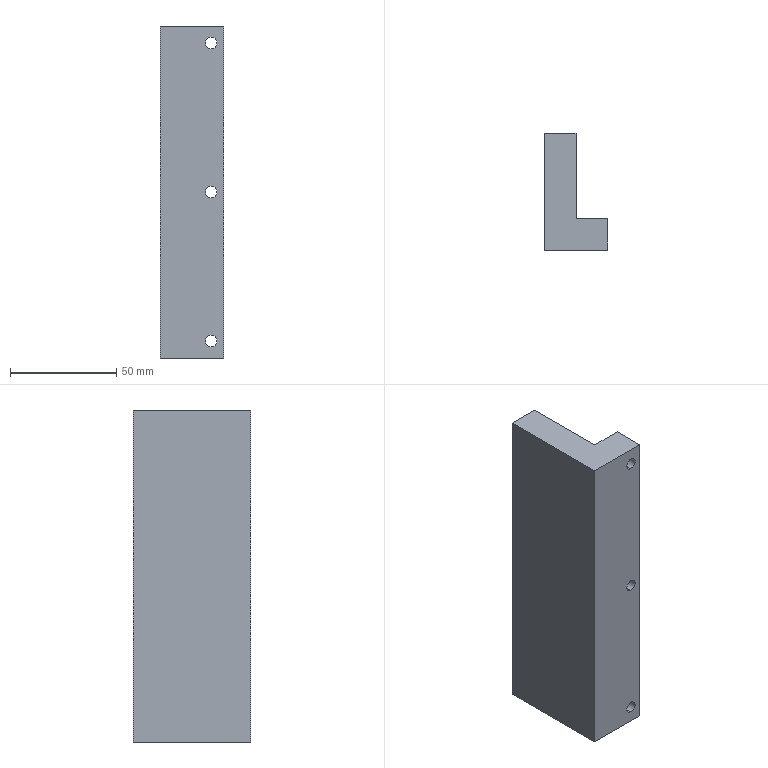Part | SolidWorks | features 3DProfileFeature 1, Cut 1, Extrusion 1, HoleWzd 1 | 1 solid | 26 faces | box 30 x 55 x 156 mm | volume 162115 mm3 | cylinder 12 | plane 8 | cone 6 | commonest cylinder face diameters 4.2 x6 5.5 x6
STEP:
#1=CARTESIAN_POINT('',(24.,0.,67.25));
#2=VERTEX_POINT('',#1);
#3=CARTESIAN_POINT('',(24.,0.,72.75));
#4=VERTEX_POINT('',#3);
#5=CARTESIAN_POINT('',(24.,0.,70.));
#6=DIRECTION('',(0.,1.,0.));
#7=DIRECTION('',(0.,0.,-1.));
#8=AXIS2_PLACEMENT_3D('',#5,#6,#7);
#9=CIRCLE('',#8,2.75);
#10=EDGE_CURVE('',#2,#4,#9,.T.);
#11=ORIENTED_EDGE('',*,*,#10,.F.);
#12=CARTESIAN_POINT('',(24.,15.,67.25));
#13=VERTEX_POINT('',#12);
#14=CARTESIAN_POINT('',(24.,0.,67.25));
#15=DIRECTION('',(0.,1.,0.));
#16=VECTOR('',#15,1000.);
#17=LINE('',#14,#16);
#18=EDGE_CURVE('',#2,#13,#17,.T.);
#19=ORIENTED_EDGE('',*,*,#18,.T.);
#20=CARTESIAN_POINT('',(24.,15.,72.75));
#21=VERTEX_POINT('',#20);
#22=CARTESIAN_POINT('',(24.,15.,70.));
#23=DIRECTION('',(0.,1.,0.));
#24=DIRECTION('',(0.,0.,-1.));
#25=AXIS2_PLACEMENT_3D('',#22,#23,#24);
#26=CIRCLE('',#25,2.75);
#27=EDGE_CURVE('',#13,#21,#26,.T.);
#28=ORIENTED_EDGE('',*,*,#27,.T.);
#29=CARTESIAN_POINT('',(24.,0.,72.75));
#30=DIRECTION('',(0.,1.,0.));
#31=VECTOR('',#30,1000.);
#32=LINE('',#29,#31);
#33=EDGE_CURVE('',#4,#21,#32,.T.);
#34=ORIENTED_EDGE('',*,*,#33,.F.);
#35=EDGE_LOOP('',(#11,#19,#28,#34));
#36=FACE_OUTER_BOUND('',#35,.T.);
#37=CARTESIAN_POINT('',(24.,0.,70.));
#38=DIRECTION('',(0.,1.,0.));
#39=DIRECTION('',(0.,0.,1.));
#40=AXIS2_PLACEMENT_3D('',#37,#38,#39);
#41=CYLINDRICAL_SURFACE('',#40,2.75);
#42=ADVANCED_FACE('',(#36),#41,.F.);
#43=CARTESIAN_POINT('',(24.,0.,-72.75));
#44=VERTEX_POINT('',#43);
#45=CARTESIAN_POINT('',(24.,0.,-67.25));
#46=VERTEX_POINT('',#45);
#47=CARTESIAN_POINT('',(24.,0.,-70.));
#48=DIRECTION('',(0.,1.,0.));
#49=DIRECTION('',(0.,0.,1.));
#50=AXIS2_PLACEMENT_3D('',#47,#48,#49);
#51=CIRCLE('',#50,2.75);
#52=EDGE_CURVE('',#44,#46,#51,.T.);
#53=ORIENTED_EDGE('',*,*,#52,.F.);
#54=CARTESIAN_POINT('',(24.,15.,-72.75));
#55=VERTEX_POINT('',#54);
#56=CARTESIAN_POINT('',(24.,0.,-72.75));
#57=DIRECTION('',(0.,1.,0.));
#58=VECTOR('',#57,1000.);
#59=LINE('',#56,#58);
#60=EDGE_CURVE('',#44,#55,#59,.T.);
#61=ORIENTED_EDGE('',*,*,#60,.T.);
#62=CARTESIAN_POINT('',(24.,15.,-67.25));
#63=VERTEX_POINT('',#62);
#64=CARTESIAN_POINT('',(24.,15.,-70.));
#65=DIRECTION('',(0.,1.,0.));
#66=DIRECTION('',(0.,0.,1.));
#67=AXIS2_PLACEMENT_3D('',#64,#65,#66);
#68=CIRCLE('',#67,2.75);
#69=EDGE_CURVE('',#55,#63,#68,.T.);
#70=ORIENTED_EDGE('',*,*,#69,.T.);
#71=CARTESIAN_POINT('',(24.,0.,-67.25));
#72=DIRECTION('',(0.,1.,0.));
#73=VECTOR('',#72,1000.);
#74=LINE('',#71,#73);
#75=EDGE_CURVE('',#46,#63,#74,.T.);
#76=ORIENTED_EDGE('',*,*,#75,.F.);
#77=EDGE_LOOP('',(#53,#61,#70,#76));
#78=FACE_OUTER_BOUND('',#77,.T.);
#79=CARTESIAN_POINT('',(24.,0.,-70.));
#80=DIRECTION('',(0.,1.,0.));
#81=DIRECTION('',(0.,0.,1.));
#82=AXIS2_PLACEMENT_3D('',#79,#80,#81);
#83=CYLINDRICAL_SURFACE('',#82,2.75);
#84=ADVANCED_FACE('',(#78),#83,.F.);
#85=CARTESIAN_POINT('',(24.,0.,-2.75));
#86=VERTEX_POINT('',#85);
#87=CARTESIAN_POINT('',(24.,0.,2.75));
#88=VERTEX_POINT('',#87);
#89=CARTESIAN_POINT('',(24.,0.,0.));
#90=DIRECTION('',(0.,1.,0.));
#91=DIRECTION('',(0.,0.,1.));
#92=AXIS2_PLACEMENT_3D('',#89,#90,#91);
#93=CIRCLE('',#92,2.75);
#94=EDGE_CURVE('',#86,#88,#93,.T.);
#95=ORIENTED_EDGE('',*,*,#94,.F.);
#96=CARTESIAN_POINT('',(24.,15.,-2.75));
#97=VERTEX_POINT('',#96);
#98=CARTESIAN_POINT('',(24.,0.,-2.75));
#99=DIRECTION('',(0.,1.,0.));
#100=VECTOR('',#99,1000.);
#101=LINE('',#98,#100);
#102=EDGE_CURVE('',#86,#97,#101,.T.);
#103=ORIENTED_EDGE('',*,*,#102,.T.);
#104=CARTESIAN_POINT('',(24.,15.,2.75));
#105=VERTEX_POINT('',#104);
#106=CARTESIAN_POINT('',(24.,15.,0.));
#107=DIRECTION('',(0.,1.,0.));
#108=DIRECTION('',(0.,0.,1.));
#109=AXIS2_PLACEMENT_3D('',#106,#107,#108);
#110=CIRCLE('',#109,2.75);
#111=EDGE_CURVE('',#97,#105,#110,.T.);
#112=ORIENTED_EDGE('',*,*,#111,.T.);
#113=CARTESIAN_POINT('',(24.,0.,2.75));
#114=DIRECTION('',(0.,1.,0.));
#115=VECTOR('',#114,1000.);
#116=LINE('',#113,#115);
#117=EDGE_CURVE('',#88,#105,#116,.T.);
#118=ORIENTED_EDGE('',*,*,#117,.F.);
#119=EDGE_LOOP('',(#95,#103,#112,#118));
#120=FACE_OUTER_BOUND('',#119,.T.);
#121=CARTESIAN_POINT('',(24.,0.,0.));
#122=DIRECTION('',(0.,1.,0.));
#123=DIRECTION('',(0.,0.,1.));
#124=AXIS2_PLACEMENT_3D('',#121,#122,#123);
#125=CYLINDRICAL_SURFACE('',#124,2.75);
#126=ADVANCED_FACE('',(#120),#125,.F.);
#127=CARTESIAN_POINT('',(7.5,39.338,0.));
#128=VERTEX_POINT('',#127);
#129=CARTESIAN_POINT('',(7.5,40.6,2.1));
#130=VERTEX_POINT('',#129);
#131=CARTESIAN_POINT('',(7.5,40.6,2.1));
#132=DIRECTION('',(0.,0.515,0.8572));
#133=VECTOR('',#132,1000.);
#134=LINE('',#131,#133);
#135=EDGE_CURVE('',#128,#130,#134,.T.);
#136=ORIENTED_EDGE('',*,*,#135,.F.);
#137=CARTESIAN_POINT('',(7.5,40.6,-2.1));
#138=VERTEX_POINT('',#137);
#139=CARTESIAN_POINT('',(7.5,40.6,-2.1));
#140=DIRECTION('',(0.,0.515,-0.8572));
#141=VECTOR('',#140,1000.);
#142=LINE('',#139,#141);
#143=EDGE_CURVE('',#128,#138,#142,.T.);
#144=ORIENTED_EDGE('',*,*,#143,.T.);
#145=CARTESIAN_POINT('',(7.5,40.6,0.));
#146=DIRECTION('',(0.,1.,0.));
#147=DIRECTION('',(0.,0.,1.));
#148=AXIS2_PLACEMENT_3D('',#145,#146,#147);
#149=CIRCLE('',#148,2.1);
#150=EDGE_CURVE('',#138,#130,#149,.T.);
#151=ORIENTED_EDGE('',*,*,#150,.T.);
#152=EDGE_LOOP('',(#136,#144,#151));
#153=FACE_OUTER_BOUND('',#152,.T.);
#154=CARTESIAN_POINT('',(7.5,40.6,0.));
#155=DIRECTION('',(0.,1.,0.));
#156=DIRECTION('',(0.,0.,1.));
#157=AXIS2_PLACEMENT_3D('',#154,#155,#156);
#158=CONICAL_SURFACE('',#157,2.1,1.03);
#159=ADVANCED_FACE('',(#153),#158,.F.);
#160=ORIENTED_EDGE('',*,*,#150,.F.);
#161=CARTESIAN_POINT('',(7.5,55.,-2.1));
#162=VERTEX_POINT('',#161);
#163=CARTESIAN_POINT('',(7.5,55.,-2.1));
#164=DIRECTION('',(0.,1.,0.));
#165=VECTOR('',#164,1000.);
#166=LINE('',#163,#165);
#167=EDGE_CURVE('',#138,#162,#166,.T.);
#168=ORIENTED_EDGE('',*,*,#167,.T.);
#169=CARTESIAN_POINT('',(7.5,55.,2.1));
#170=VERTEX_POINT('',#169);
#171=CARTESIAN_POINT('',(7.5,55.,0.));
#172=DIRECTION('',(0.,1.,0.));
#173=DIRECTION('',(0.,0.,1.));
#174=AXIS2_PLACEMENT_3D('',#171,#172,#173);
#175=CIRCLE('',#174,2.1);
#176=EDGE_CURVE('',#162,#170,#175,.T.);
#177=ORIENTED_EDGE('',*,*,#176,.T.);
#178=CARTESIAN_POINT('',(7.5,55.,2.1));
#179=DIRECTION('',(0.,1.,0.));
#180=VECTOR('',#179,1000.);
#181=LINE('',#178,#180);
#182=EDGE_CURVE('',#130,#170,#181,.T.);
#183=ORIENTED_EDGE('',*,*,#182,.F.);
#184=EDGE_LOOP('',(#160,#168,#177,#183));
#185=FACE_OUTER_BOUND('',#184,.T.);
#186=CARTESIAN_POINT('',(7.5,55.,0.));
#187=DIRECTION('',(0.,1.,0.));
#188=DIRECTION('',(0.,0.,1.));
#189=AXIS2_PLACEMENT_3D('',#186,#187,#188);
#190=CYLINDRICAL_SURFACE('',#189,2.1);
#191=ADVANCED_FACE('',(#185),#190,.F.);
#192=CARTESIAN_POINT('',(7.5,39.338,-70.));
#193=VERTEX_POINT('',#192);
#194=CARTESIAN_POINT('',(7.5,40.6,-67.9));
#195=VERTEX_POINT('',#194);
#196=CARTESIAN_POINT('',(7.5,40.6,-67.9));
#197=DIRECTION('',(0.,0.515,0.8572));
#198=VECTOR('',#197,1000.);
#199=LINE('',#196,#198);
#200=EDGE_CURVE('',#193,#195,#199,.T.);
#201=ORIENTED_EDGE('',*,*,#200,.F.);
#202=CARTESIAN_POINT('',(7.5,40.6,-72.1));
#203=VERTEX_POINT('',#202);
#204=CARTESIAN_POINT('',(7.5,40.6,-72.1));
#205=DIRECTION('',(0.,0.515,-0.8572));
#206=VECTOR('',#205,1000.);
#207=LINE('',#204,#206);
#208=EDGE_CURVE('',#193,#203,#207,.T.);
#209=ORIENTED_EDGE('',*,*,#208,.T.);
#210=CARTESIAN_POINT('',(7.5,40.6,-70.));
#211=DIRECTION('',(0.,1.,0.));
#212=DIRECTION('',(0.,0.,1.));
#213=AXIS2_PLACEMENT_3D('',#210,#211,#212);
#214=CIRCLE('',#213,2.1);
#215=EDGE_CURVE('',#203,#195,#214,.T.);
#216=ORIENTED_EDGE('',*,*,#215,.T.);
#217=EDGE_LOOP('',(#201,#209,#216));
#218=FACE_OUTER_BOUND('',#217,.T.);
#219=CARTESIAN_POINT('',(7.5,40.6,-70.));
#220=DIRECTION('',(0.,1.,0.));
#221=DIRECTION('',(0.,0.,1.));
#222=AXIS2_PLACEMENT_3D('',#219,#220,#221);
#223=CONICAL_SURFACE('',#222,2.1,1.03);
#224=ADVANCED_FACE('',(#218),#223,.F.);
#225=ORIENTED_EDGE('',*,*,#215,.F.);
#226=CARTESIAN_POINT('',(7.5,55.,-72.1));
#227=VERTEX_POINT('',#226);
#228=CARTESIAN_POINT('',(7.5,55.,-72.1));
#229=DIRECTION('',(0.,1.,0.));
#230=VECTOR('',#229,1000.);
#231=LINE('',#228,#230);
#232=EDGE_CURVE('',#203,#227,#231,.T.);
#233=ORIENTED_EDGE('',*,*,#232,.T.);
#234=CARTESIAN_POINT('',(7.5,55.,-67.9));
#235=VERTEX_POINT('',#234);
#236=CARTESIAN_POINT('',(7.5,55.,-70.));
#237=DIRECTION('',(0.,1.,0.));
#238=DIRECTION('',(0.,0.,1.));
#239=AXIS2_PLACEMENT_3D('',#236,#237,#238);
#240=CIRCLE('',#239,2.1);
#241=EDGE_CURVE('',#227,#235,#240,.T.);
#242=ORIENTED_EDGE('',*,*,#241,.T.);
#243=CARTESIAN_POINT('',(7.5,55.,-67.9));
#244=DIRECTION('',(0.,1.,0.));
#245=VECTOR('',#244,1000.);
#246=LINE('',#243,#245);
#247=EDGE_CURVE('',#195,#235,#246,.T.);
#248=ORIENTED_EDGE('',*,*,#247,.F.);
#249=EDGE_LOOP('',(#225,#233,#242,#248));
#250=FACE_OUTER_BOUND('',#249,.T.);
#251=CARTESIAN_POINT('',(7.5,55.,-70.));
#252=DIRECTION('',(0.,1.,0.));
#253=DIRECTION('',(0.,0.,1.));
#254=AXIS2_PLACEMENT_3D('',#251,#252,#253);
#255=CYLINDRICAL_SURFACE('',#254,2.1);
#256=ADVANCED_FACE('',(#250),#255,.F.);
#257=CARTESIAN_POINT('',(7.5,39.338,70.));
#258=VERTEX_POINT('',#257);
#259=CARTESIAN_POINT('',(7.5,40.6,72.1));
#260=VERTEX_POINT('',#259);
#261=CARTESIAN_POINT('',(7.5,40.6,72.1));
#262=DIRECTION('',(0.,0.515,0.8572));
#263=VECTOR('',#262,1000.);
#264=LINE('',#261,#263);
#265=EDGE_CURVE('',#258,#260,#264,.T.);
#266=ORIENTED_EDGE('',*,*,#265,.F.);
#267=CARTESIAN_POINT('',(7.5,40.6,67.9));
#268=VERTEX_POINT('',#267);
#269=CARTESIAN_POINT('',(7.5,40.6,67.9));
#270=DIRECTION('',(0.,0.515,-0.8572));
#271=VECTOR('',#270,1000.);
#272=LINE('',#269,#271);
#273=EDGE_CURVE('',#258,#268,#272,.T.);
#274=ORIENTED_EDGE('',*,*,#273,.T.);
#275=CARTESIAN_POINT('',(7.5,40.6,70.));
#276=DIRECTION('',(0.,1.,0.));
#277=DIRECTION('',(0.,0.,1.));
#278=AXIS2_PLACEMENT_3D('',#275,#276,#277);
#279=CIRCLE('',#278,2.1);
#280=EDGE_CURVE('',#268,#260,#279,.T.);
#281=ORIENTED_EDGE('',*,*,#280,.T.);
#282=EDGE_LOOP('',(#266,#274,#281));
#283=FACE_OUTER_BOUND('',#282,.T.);
#284=CARTESIAN_POINT('',(7.5,40.6,70.));
#285=DIRECTION('',(0.,1.,0.));
#286=DIRECTION('',(0.,0.,1.));
#287=AXIS2_PLACEMENT_3D('',#284,#285,#286);
#288=CONICAL_SURFACE('',#287,2.1,1.03);
#289=ADVANCED_FACE('',(#283),#288,.F.);
#290=ORIENTED_EDGE('',*,*,#280,.F.);
#291=CARTESIAN_POINT('',(7.5,55.,67.9));
#292=VERTEX_POINT('',#291);
#293=CARTESIAN_POINT('',(7.5,55.,67.9));
#294=DIRECTION('',(0.,1.,0.));
#295=VECTOR('',#294,1000.);
#296=LINE('',#293,#295);
#297=EDGE_CURVE('',#268,#292,#296,.T.);
#298=ORIENTED_EDGE('',*,*,#297,.T.);
#299=CARTESIAN_POINT('',(7.5,55.,72.1));
#300=VERTEX_POINT('',#299);
#301=CARTESIAN_POINT('',(7.5,55.,70.));
#302=DIRECTION('',(0.,1.,0.));
#303=DIRECTION('',(0.,0.,1.));
#304=AXIS2_PLACEMENT_3D('',#301,#302,#303);
#305=CIRCLE('',#304,2.1);
#306=EDGE_CURVE('',#292,#300,#305,.T.);
#307=ORIENTED_EDGE('',*,*,#306,.T.);
#308=CARTESIAN_POINT('',(7.5,55.,72.1));
#309=DIRECTION('',(0.,1.,0.));
#310=VECTOR('',#309,1000.);
#311=LINE('',#308,#310);
#312=EDGE_CURVE('',#260,#300,#311,.T.);
#313=ORIENTED_EDGE('',*,*,#312,.F.);
#314=EDGE_LOOP('',(#290,#298,#307,#313));
#315=FACE_OUTER_BOUND('',#314,.T.);
#316=CARTESIAN_POINT('',(7.5,55.,70.));
#317=DIRECTION('',(0.,1.,0.));
#318=DIRECTION('',(0.,0.,1.));
#319=AXIS2_PLACEMENT_3D('',#316,#317,#318);
#320=CYLINDRICAL_SURFACE('',#319,2.1);
#321=ADVANCED_FACE('',(#315),#320,.F.);
#322=CARTESIAN_POINT('',(7.5,55.,0.));
#323=DIRECTION('',(0.,1.,0.));
#324=DIRECTION('',(0.,0.,1.));
#325=AXIS2_PLACEMENT_3D('',#322,#323,#324);
#326=CIRCLE('',#325,2.1);
#327=EDGE_CURVE('',#170,#162,#326,.T.);
#328=ORIENTED_EDGE('',*,*,#327,.F.);
#329=ORIENTED_EDGE('',*,*,#176,.F.);
#330=EDGE_LOOP('',(#328,#329));
#331=FACE_BOUND('',#330,.T.);
#332=CARTESIAN_POINT('',(7.5,55.,-70.));
#333=DIRECTION('',(0.,1.,0.));
#334=DIRECTION('',(0.,0.,1.));
#335=AXIS2_PLACEMENT_3D('',#332,#333,#334);
#336=CIRCLE('',#335,2.1);
#337=EDGE_CURVE('',#235,#227,#336,.T.);
#338=ORIENTED_EDGE('',*,*,#337,.F.);
#339=ORIENTED_EDGE('',*,*,#241,.F.);
#340=EDGE_LOOP('',(#338,#339));
#341=FACE_BOUND('',#340,.T.);
#342=CARTESIAN_POINT('',(7.5,55.,70.));
#343=DIRECTION('',(0.,1.,0.));
#344=DIRECTION('',(0.,0.,1.));
#345=AXIS2_PLACEMENT_3D('',#342,#343,#344);
#346=CIRCLE('',#345,2.1);
#347=EDGE_CURVE('',#300,#292,#346,.T.);
#348=ORIENTED_EDGE('',*,*,#347,.F.);
#349=ORIENTED_EDGE('',*,*,#306,.F.);
#350=EDGE_LOOP('',(#348,#349));
#351=FACE_BOUND('',#350,.T.);
#352=CARTESIAN_POINT('',(15.,55.,-78.));
#353=VERTEX_POINT('',#352);
#354=CARTESIAN_POINT('',(0.,55.,-78.));
#355=VERTEX_POINT('',#354);
#356=CARTESIAN_POINT('',(15.,55.,-78.));
#357=DIRECTION('',(-1.,0.,0.));
#358=VECTOR('',#357,1000.);
#359=LINE('',#356,#358);
#360=EDGE_CURVE('',#353,#355,#359,.T.);
#361=ORIENTED_EDGE('',*,*,#360,.T.);
#362=CARTESIAN_POINT('',(0.,55.,78.));
#363=VERTEX_POINT('',#362);
#364=CARTESIAN_POINT('',(0.,55.,78.));
#365=DIRECTION('',(0.,0.,-1.));
#366=VECTOR('',#365,1000.);
#367=LINE('',#364,#366);
#368=EDGE_CURVE('',#363,#355,#367,.T.);
#369=ORIENTED_EDGE('',*,*,#368,.F.);
#370=CARTESIAN_POINT('',(15.,55.,78.));
#371=VERTEX_POINT('',#370);
#372=CARTESIAN_POINT('',(15.,55.,78.));
#373=DIRECTION('',(-1.,0.,0.));
#374=VECTOR('',#373,1000.);
#375=LINE('',#372,#374);
#376=EDGE_CURVE('',#371,#363,#375,.T.);
#377=ORIENTED_EDGE('',*,*,#376,.F.);
#378=CARTESIAN_POINT('',(15.,55.,78.));
#379=DIRECTION('',(0.,0.,-1.));
#380=VECTOR('',#379,1000.);
#381=LINE('',#378,#380);
#382=EDGE_CURVE('',#371,#353,#381,.T.);
#383=ORIENTED_EDGE('',*,*,#382,.T.);
#384=EDGE_LOOP('',(#361,#369,#377,#383));
#385=FACE_OUTER_BOUND('',#384,.T.);
#386=CARTESIAN_POINT('',(15.,55.,78.));
#387=DIRECTION('',(0.,-1.,0.));
#388=DIRECTION('',(0.,0.,-1.));
#389=AXIS2_PLACEMENT_3D('',#386,#387,#388);
#390=PLANE('',#389);
#391=ADVANCED_FACE('',(#331,#341,#351,#385),#390,.F.);
#392=CARTESIAN_POINT('',(0.,0.,-78.));
#393=VERTEX_POINT('',#392);
#394=CARTESIAN_POINT('',(0.,55.,-78.));
#395=DIRECTION('',(0.,-1.,0.));
#396=VECTOR('',#395,1000.);
#397=LINE('',#394,#396);
#398=EDGE_CURVE('',#355,#393,#397,.T.);
#399=ORIENTED_EDGE('',*,*,#398,.T.);
#400=CARTESIAN_POINT('',(0.,0.,78.));
#401=VERTEX_POINT('',#400);
#402=CARTESIAN_POINT('',(0.,0.,78.));
#403=DIRECTION('',(0.,0.,-1.));
#404=VECTOR('',#403,1000.);
#405=LINE('',#402,#404);
#406=EDGE_CURVE('',#401,#393,#405,.T.);
#407=ORIENTED_EDGE('',*,*,#406,.F.);
#408=CARTESIAN_POINT('',(0.,55.,78.));
#409=DIRECTION('',(0.,-1.,0.));
#410=VECTOR('',#409,1000.);
#411=LINE('',#408,#410);
#412=EDGE_CURVE('',#363,#401,#411,.T.);
#413=ORIENTED_EDGE('',*,*,#412,.F.);
#414=ORIENTED_EDGE('',*,*,#368,.T.);
#415=EDGE_LOOP('',(#399,#407,#413,#414));
#416=FACE_OUTER_BOUND('',#415,.T.);
#417=CARTESIAN_POINT('',(0.,55.,78.));
#418=DIRECTION('',(1.,0.,0.));
#419=DIRECTION('',(0.,1.,0.));
#420=AXIS2_PLACEMENT_3D('',#417,#418,#419);
#421=PLANE('',#420);
#422=ADVANCED_FACE('',(#416),#421,.F.);
#423=CARTESIAN_POINT('',(24.,0.,70.));
#424=DIRECTION('',(0.,1.,0.));
#425=DIRECTION('',(0.,0.,-1.));
#426=AXIS2_PLACEMENT_3D('',#423,#424,#425);
#427=CIRCLE('',#426,2.75);
#428=EDGE_CURVE('',#4,#2,#427,.T.);
#429=ORIENTED_EDGE('',*,*,#428,.T.);
#430=ORIENTED_EDGE('',*,*,#10,.T.);
#431=EDGE_LOOP('',(#429,#430));
#432=FACE_BOUND('',#431,.T.);
#433=CARTESIAN_POINT('',(24.,0.,-70.));
#434=DIRECTION('',(0.,1.,0.));
#435=DIRECTION('',(0.,0.,1.));
#436=AXIS2_PLACEMENT_3D('',#433,#434,#435);
#437=CIRCLE('',#436,2.75);
#438=EDGE_CURVE('',#46,#44,#437,.T.);
#439=ORIENTED_EDGE('',*,*,#438,.T.);
#440=ORIENTED_EDGE('',*,*,#52,.T.);
#441=EDGE_LOOP('',(#439,#440));
#442=FACE_BOUND('',#441,.T.);
#443=CARTESIAN_POINT('',(24.,0.,0.));
#444=DIRECTION('',(0.,1.,0.));
#445=DIRECTION('',(0.,0.,1.));
#446=AXIS2_PLACEMENT_3D('',#443,#444,#445);
#447=CIRCLE('',#446,2.75);
#448=EDGE_CURVE('',#88,#86,#447,.T.);
#449=ORIENTED_EDGE('',*,*,#448,.T.);
#450=ORIENTED_EDGE('',*,*,#94,.T.);
#451=EDGE_LOOP('',(#449,#450));
#452=FACE_BOUND('',#451,.T.);
#453=CARTESIAN_POINT('',(30.,0.,-78.));
#454=VERTEX_POINT('',#453);
#455=CARTESIAN_POINT('',(0.,0.,-78.));
#456=DIRECTION('',(1.,0.,0.));
#457=VECTOR('',#456,1000.);
#458=LINE('',#455,#457);
#459=EDGE_CURVE('',#393,#454,#458,.T.);
#460=ORIENTED_EDGE('',*,*,#459,.T.);
#461=CARTESIAN_POINT('',(30.,0.,78.));
#462=VERTEX_POINT('',#461);
#463=CARTESIAN_POINT('',(30.,0.,78.));
#464=DIRECTION('',(0.,0.,-1.));
#465=VECTOR('',#464,1000.);
#466=LINE('',#463,#465);
#467=EDGE_CURVE('',#462,#454,#466,.T.);
#468=ORIENTED_EDGE('',*,*,#467,.F.);
#469=CARTESIAN_POINT('',(0.,0.,78.));
#470=DIRECTION('',(1.,0.,0.));
#471=VECTOR('',#470,1000.);
#472=LINE('',#469,#471);
#473=EDGE_CURVE('',#401,#462,#472,.T.);
#474=ORIENTED_EDGE('',*,*,#473,.F.);
#475=ORIENTED_EDGE('',*,*,#406,.T.);
#476=EDGE_LOOP('',(#460,#468,#474,#475));
#477=FACE_OUTER_BOUND('',#476,.T.);
#478=CARTESIAN_POINT('',(0.,0.,78.));
#479=DIRECTION('',(0.,1.,0.));
#480=DIRECTION('',(0.,0.,1.));
#481=AXIS2_PLACEMENT_3D('',#478,#479,#480);
#482=PLANE('',#481);
#483=ADVANCED_FACE('',(#432,#442,#452,#477),#482,.F.);
#484=CARTESIAN_POINT('',(30.,15.,-78.));
#485=VERTEX_POINT('',#484);
#486=CARTESIAN_POINT('',(30.,0.,-78.));
#487=DIRECTION('',(0.,1.,0.));
#488=VECTOR('',#487,1000.);
#489=LINE('',#486,#488);
#490=EDGE_CURVE('',#454,#485,#489,.T.);
#491=ORIENTED_EDGE('',*,*,#490,.T.);
#492=CARTESIAN_POINT('',(30.,15.,78.));
#493=VERTEX_POINT('',#492);
#494=CARTESIAN_POINT('',(30.,15.,78.));
#495=DIRECTION('',(0.,0.,-1.));
#496=VECTOR('',#495,1000.);
#497=LINE('',#494,#496);
#498=EDGE_CURVE('',#493,#485,#497,.T.);
#499=ORIENTED_EDGE('',*,*,#498,.F.);
#500=CARTESIAN_POINT('',(30.,0.,78.));
#501=DIRECTION('',(0.,1.,0.));
#502=VECTOR('',#501,1000.);
#503=LINE('',#500,#502);
#504=EDGE_CURVE('',#462,#493,#503,.T.);
#505=ORIENTED_EDGE('',*,*,#504,.F.);
#506=ORIENTED_EDGE('',*,*,#467,.T.);
#507=EDGE_LOOP('',(#491,#499,#505,#506));
#508=FACE_OUTER_BOUND('',#507,.T.);
#509=CARTESIAN_POINT('',(30.,0.,78.));
#510=DIRECTION('',(-1.,0.,0.));
#511=DIRECTION('',(0.,0.,1.));
#512=AXIS2_PLACEMENT_3D('',#509,#510,#511);
#513=PLANE('',#512);
#514=ADVANCED_FACE('',(#508),#513,.F.);
#515=CARTESIAN_POINT('',(24.,15.,70.));
#516=DIRECTION('',(0.,1.,0.));
#517=DIRECTION('',(0.,0.,-1.));
#518=AXIS2_PLACEMENT_3D('',#515,#516,#517);
#519=CIRCLE('',#518,2.75);
#520=EDGE_CURVE('',#21,#13,#519,.T.);
#521=ORIENTED_EDGE('',*,*,#520,.F.);
#522=ORIENTED_EDGE('',*,*,#27,.F.);
#523=EDGE_LOOP('',(#521,#522));
#524=FACE_BOUND('',#523,.T.);
#525=CARTESIAN_POINT('',(24.,15.,-70.));
#526=DIRECTION('',(0.,1.,0.));
#527=DIRECTION('',(0.,0.,1.));
#528=AXIS2_PLACEMENT_3D('',#525,#526,#527);
#529=CIRCLE('',#528,2.75);
#530=EDGE_CURVE('',#63,#55,#529,.T.);
#531=ORIENTED_EDGE('',*,*,#530,.F.);
#532=ORIENTED_EDGE('',*,*,#69,.F.);
#533=EDGE_LOOP('',(#531,#532));
#534=FACE_BOUND('',#533,.T.);
#535=CARTESIAN_POINT('',(24.,15.,0.));
#536=DIRECTION('',(0.,1.,0.));
#537=DIRECTION('',(0.,0.,1.));
#538=AXIS2_PLACEMENT_3D('',#535,#536,#537);
#539=CIRCLE('',#538,2.75);
#540=EDGE_CURVE('',#105,#97,#539,.T.);
#541=ORIENTED_EDGE('',*,*,#540,.F.);
#542=ORIENTED_EDGE('',*,*,#111,.F.);
#543=EDGE_LOOP('',(#541,#542));
#544=FACE_BOUND('',#543,.T.);
#545=CARTESIAN_POINT('',(15.,15.,-78.));
#546=VERTEX_POINT('',#545);
#547=CARTESIAN_POINT('',(30.,15.,-78.));
#548=DIRECTION('',(-1.,0.,0.));
#549=VECTOR('',#548,1000.);
#550=LINE('',#547,#549);
#551=EDGE_CURVE('',#485,#546,#550,.T.);
#552=ORIENTED_EDGE('',*,*,#551,.T.);
#553=CARTESIAN_POINT('',(15.,15.,78.));
#554=VERTEX_POINT('',#553);
#555=CARTESIAN_POINT('',(15.,15.,78.));
#556=DIRECTION('',(0.,0.,-1.));
#557=VECTOR('',#556,1000.);
#558=LINE('',#555,#557);
#559=EDGE_CURVE('',#554,#546,#558,.T.);
#560=ORIENTED_EDGE('',*,*,#559,.F.);
#561=CARTESIAN_POINT('',(30.,15.,78.));
#562=DIRECTION('',(-1.,0.,0.));
#563=VECTOR('',#562,1000.);
#564=LINE('',#561,#563);
#565=EDGE_CURVE('',#493,#554,#564,.T.);
#566=ORIENTED_EDGE('',*,*,#565,.F.);
#567=ORIENTED_EDGE('',*,*,#498,.T.);
#568=EDGE_LOOP('',(#552,#560,#566,#567));
#569=FACE_OUTER_BOUND('',#568,.T.);
#570=CARTESIAN_POINT('',(30.,15.,78.));
#571=DIRECTION('',(0.,-1.,0.));
#572=DIRECTION('',(0.,0.,-1.));
#573=AXIS2_PLACEMENT_3D('',#570,#571,#572);
#574=PLANE('',#573);
#575=ADVANCED_FACE('',(#524,#534,#544,#569),#574,.F.);
#576=CARTESIAN_POINT('',(15.,15.,-78.));
#577=DIRECTION('',(0.,1.,0.));
#578=VECTOR('',#577,1000.);
#579=LINE('',#576,#578);
#580=EDGE_CURVE('',#546,#353,#579,.T.);
#581=ORIENTED_EDGE('',*,*,#580,.T.);
#582=ORIENTED_EDGE('',*,*,#382,.F.);
#583=CARTESIAN_POINT('',(15.,15.,78.));
#584=DIRECTION('',(0.,1.,0.));
#585=VECTOR('',#584,1000.);
#586=LINE('',#583,#585);
#587=EDGE_CURVE('',#554,#371,#586,.T.);
#588=ORIENTED_EDGE('',*,*,#587,.F.);
#589=ORIENTED_EDGE('',*,*,#559,.T.);
#590=EDGE_LOOP('',(#581,#582,#588,#589));
#591=FACE_OUTER_BOUND('',#590,.T.);
#592=CARTESIAN_POINT('',(15.,15.,78.));
#593=DIRECTION('',(-1.,0.,0.));
#594=DIRECTION('',(0.,0.,1.));
#595=AXIS2_PLACEMENT_3D('',#592,#593,#594);
#596=PLANE('',#595);
#597=ADVANCED_FACE('',(#591),#596,.F.);
#598=ORIENTED_EDGE('',*,*,#376,.T.);
#599=ORIENTED_EDGE('',*,*,#412,.T.);
#600=ORIENTED_EDGE('',*,*,#473,.T.);
#601=ORIENTED_EDGE('',*,*,#504,.T.);
#602=ORIENTED_EDGE('',*,*,#565,.T.);
#603=ORIENTED_EDGE('',*,*,#587,.T.);
#604=EDGE_LOOP('',(#598,#599,#600,#601,#602,#603));
#605=FACE_OUTER_BOUND('',#604,.T.);
#606=CARTESIAN_POINT('',(30.,55.,78.));
#607=DIRECTION('',(0.,0.,-1.));
#608=DIRECTION('',(-1.,0.,0.));
#609=AXIS2_PLACEMENT_3D('',#606,#607,#608);
#610=PLANE('',#609);
#611=ADVANCED_FACE('',(#605),#610,.F.);
#612=ORIENTED_EDGE('',*,*,#360,.F.);
#613=ORIENTED_EDGE('',*,*,#580,.F.);
#614=ORIENTED_EDGE('',*,*,#551,.F.);
#615=ORIENTED_EDGE('',*,*,#490,.F.);
#616=ORIENTED_EDGE('',*,*,#459,.F.);
#617=ORIENTED_EDGE('',*,*,#398,.F.);
#618=EDGE_LOOP('',(#612,#613,#614,#615,#616,#617));
#619=FACE_OUTER_BOUND('',#618,.T.);
#620=CARTESIAN_POINT('',(30.,55.,-78.));
#621=DIRECTION('',(0.,0.,-1.));
#622=DIRECTION('',(-1.,0.,0.));
#623=AXIS2_PLACEMENT_3D('',#620,#621,#622);
#624=PLANE('',#623);
#625=ADVANCED_FACE('',(#619),#624,.T.);
#626=ORIENTED_EDGE('',*,*,#297,.F.);
#627=CARTESIAN_POINT('',(7.5,40.6,70.));
#628=DIRECTION('',(0.,1.,0.));
#629=DIRECTION('',(0.,0.,1.));
#630=AXIS2_PLACEMENT_3D('',#627,#628,#629);
#631=CIRCLE('',#630,2.1);
#632=EDGE_CURVE('',#260,#268,#631,.T.);
#633=ORIENTED_EDGE('',*,*,#632,.F.);
#634=ORIENTED_EDGE('',*,*,#312,.T.);
#635=ORIENTED_EDGE('',*,*,#347,.T.);
#636=EDGE_LOOP('',(#626,#633,#634,#635));
#637=FACE_OUTER_BOUND('',#636,.T.);
#638=CARTESIAN_POINT('',(7.5,55.,70.));
#639=DIRECTION('',(0.,1.,0.));
#640=DIRECTION('',(0.,0.,1.));
#641=AXIS2_PLACEMENT_3D('',#638,#639,#640);
#642=CYLINDRICAL_SURFACE('',#641,2.1);
#643=ADVANCED_FACE('',(#637),#642,.F.);
#644=ORIENTED_EDGE('',*,*,#273,.F.);
#645=ORIENTED_EDGE('',*,*,#265,.T.);
#646=ORIENTED_EDGE('',*,*,#632,.T.);
#647=EDGE_LOOP('',(#644,#645,#646));
#648=FACE_OUTER_BOUND('',#647,.T.);
#649=CARTESIAN_POINT('',(7.5,40.6,70.));
#650=DIRECTION('',(0.,1.,0.));
#651=DIRECTION('',(0.,0.,1.));
#652=AXIS2_PLACEMENT_3D('',#649,#650,#651);
#653=CONICAL_SURFACE('',#652,2.1,1.03);
#654=ADVANCED_FACE('',(#648),#653,.F.);
#655=ORIENTED_EDGE('',*,*,#232,.F.);
#656=CARTESIAN_POINT('',(7.5,40.6,-70.));
#657=DIRECTION('',(0.,1.,0.));
#658=DIRECTION('',(0.,0.,1.));
#659=AXIS2_PLACEMENT_3D('',#656,#657,#658);
#660=CIRCLE('',#659,2.1);
#661=EDGE_CURVE('',#195,#203,#660,.T.);
#662=ORIENTED_EDGE('',*,*,#661,.F.);
#663=ORIENTED_EDGE('',*,*,#247,.T.);
#664=ORIENTED_EDGE('',*,*,#337,.T.);
#665=EDGE_LOOP('',(#655,#662,#663,#664));
#666=FACE_OUTER_BOUND('',#665,.T.);
#667=CARTESIAN_POINT('',(7.5,55.,-70.));
#668=DIRECTION('',(0.,1.,0.));
#669=DIRECTION('',(0.,0.,1.));
#670=AXIS2_PLACEMENT_3D('',#667,#668,#669);
#671=CYLINDRICAL_SURFACE('',#670,2.1);
#672=ADVANCED_FACE('',(#666),#671,.F.);
#673=ORIENTED_EDGE('',*,*,#208,.F.);
#674=ORIENTED_EDGE('',*,*,#200,.T.);
#675=ORIENTED_EDGE('',*,*,#661,.T.);
#676=EDGE_LOOP('',(#673,#674,#675));
#677=FACE_OUTER_BOUND('',#676,.T.);
#678=CARTESIAN_POINT('',(7.5,40.6,-70.));
#679=DIRECTION('',(0.,1.,0.));
#680=DIRECTION('',(0.,0.,1.));
#681=AXIS2_PLACEMENT_3D('',#678,#679,#680);
#682=CONICAL_SURFACE('',#681,2.1,1.03);
#683=ADVANCED_FACE('',(#677),#682,.F.);
#684=ORIENTED_EDGE('',*,*,#167,.F.);
#685=CARTESIAN_POINT('',(7.5,40.6,0.));
#686=DIRECTION('',(0.,1.,0.));
#687=DIRECTION('',(0.,0.,1.));
#688=AXIS2_PLACEMENT_3D('',#685,#686,#687);
#689=CIRCLE('',#688,2.1);
#690=EDGE_CURVE('',#130,#138,#689,.T.);
#691=ORIENTED_EDGE('',*,*,#690,.F.);
#692=ORIENTED_EDGE('',*,*,#182,.T.);
#693=ORIENTED_EDGE('',*,*,#327,.T.);
#694=EDGE_LOOP('',(#684,#691,#692,#693));
#695=FACE_OUTER_BOUND('',#694,.T.);
#696=CARTESIAN_POINT('',(7.5,55.,0.));
#697=DIRECTION('',(0.,1.,0.));
#698=DIRECTION('',(0.,0.,1.));
#699=AXIS2_PLACEMENT_3D('',#696,#697,#698);
#700=CYLINDRICAL_SURFACE('',#699,2.1);
#701=ADVANCED_FACE('',(#695),#700,.F.);
#702=ORIENTED_EDGE('',*,*,#143,.F.);
#703=ORIENTED_EDGE('',*,*,#135,.T.);
#704=ORIENTED_EDGE('',*,*,#690,.T.);
#705=EDGE_LOOP('',(#702,#703,#704));
#706=FACE_OUTER_BOUND('',#705,.T.);
#707=CARTESIAN_POINT('',(7.5,40.6,0.));
#708=DIRECTION('',(0.,1.,0.));
#709=DIRECTION('',(0.,0.,1.));
#710=AXIS2_PLACEMENT_3D('',#707,#708,#709);
#711=CONICAL_SURFACE('',#710,2.1,1.03);
#712=ADVANCED_FACE('',(#706),#711,.F.);
#713=ORIENTED_EDGE('',*,*,#102,.F.);
#714=ORIENTED_EDGE('',*,*,#448,.F.);
#715=ORIENTED_EDGE('',*,*,#117,.T.);
#716=ORIENTED_EDGE('',*,*,#540,.T.);
#717=EDGE_LOOP('',(#713,#714,#715,#716));
#718=FACE_OUTER_BOUND('',#717,.T.);
#719=CARTESIAN_POINT('',(24.,0.,0.));
#720=DIRECTION('',(0.,1.,0.));
#721=DIRECTION('',(0.,0.,1.));
#722=AXIS2_PLACEMENT_3D('',#719,#720,#721);
#723=CYLINDRICAL_SURFACE('',#722,2.75);
#724=ADVANCED_FACE('',(#718),#723,.F.);
#725=ORIENTED_EDGE('',*,*,#60,.F.);
#726=ORIENTED_EDGE('',*,*,#438,.F.);
#727=ORIENTED_EDGE('',*,*,#75,.T.);
#728=ORIENTED_EDGE('',*,*,#530,.T.);
#729=EDGE_LOOP('',(#725,#726,#727,#728));
#730=FACE_OUTER_BOUND('',#729,.T.);
#731=CARTESIAN_POINT('',(24.,0.,-70.));
#732=DIRECTION('',(0.,1.,0.));
#733=DIRECTION('',(0.,0.,1.));
#734=AXIS2_PLACEMENT_3D('',#731,#732,#733);
#735=CYLINDRICAL_SURFACE('',#734,2.75);
#736=ADVANCED_FACE('',(#730),#735,.F.);
#737=ORIENTED_EDGE('',*,*,#18,.F.);
#738=ORIENTED_EDGE('',*,*,#428,.F.);
#739=ORIENTED_EDGE('',*,*,#33,.T.);
#740=ORIENTED_EDGE('',*,*,#520,.T.);
#741=EDGE_LOOP('',(#737,#738,#739,#740));
#742=FACE_OUTER_BOUND('',#741,.T.);
#743=CARTESIAN_POINT('',(24.,0.,70.));
#744=DIRECTION('',(0.,1.,0.));
#745=DIRECTION('',(0.,0.,1.));
#746=AXIS2_PLACEMENT_3D('',#743,#744,#745);
#747=CYLINDRICAL_SURFACE('',#746,2.75);
#748=ADVANCED_FACE('',(#742),#747,.F.);
#749=CLOSED_SHELL('',(#42,#84,#126,#159,#191,#224,#256,#289,#321,#391,#422,#483,#514,#575,#597,#611,#625,#643,#654,#672,#683,#701,#712,#724,#736,#748));
#750=MANIFOLD_SOLID_BREP('',#749);
#751=CARTESIAN_POINT('',(0.,0.,0.));
#752=DIRECTION('',(0.,0.,1.));
#753=DIRECTION('',(1.,0.,0.));
#754=AXIS2_PLACEMENT_3D('',#751,#752,#753);
#755=(LENGTH_UNIT()NAMED_UNIT(*)SI_UNIT(.MILLI.,.METRE.));
#756=UNCERTAINTY_MEASURE_WITH_UNIT(LENGTH_MEASURE(0.00001),#755,'','');
#757=(NAMED_UNIT(*)PLANE_ANGLE_UNIT()SI_UNIT($,.RADIAN.));
#758=(NAMED_UNIT(*)SI_UNIT($,.STERADIAN.)SOLID_ANGLE_UNIT());
#759=(GEOMETRIC_REPRESENTATION_CONTEXT(3)GLOBAL_UNCERTAINTY_ASSIGNED_CONTEXT((#756))GLOBAL_UNIT_ASSIGNED_CONTEXT((#755,#757,#758))REPRESENTATION_CONTEXT('',''));
#760=ADVANCED_BREP_SHAPE_REPRESENTATION('',(#750,#754),#759);